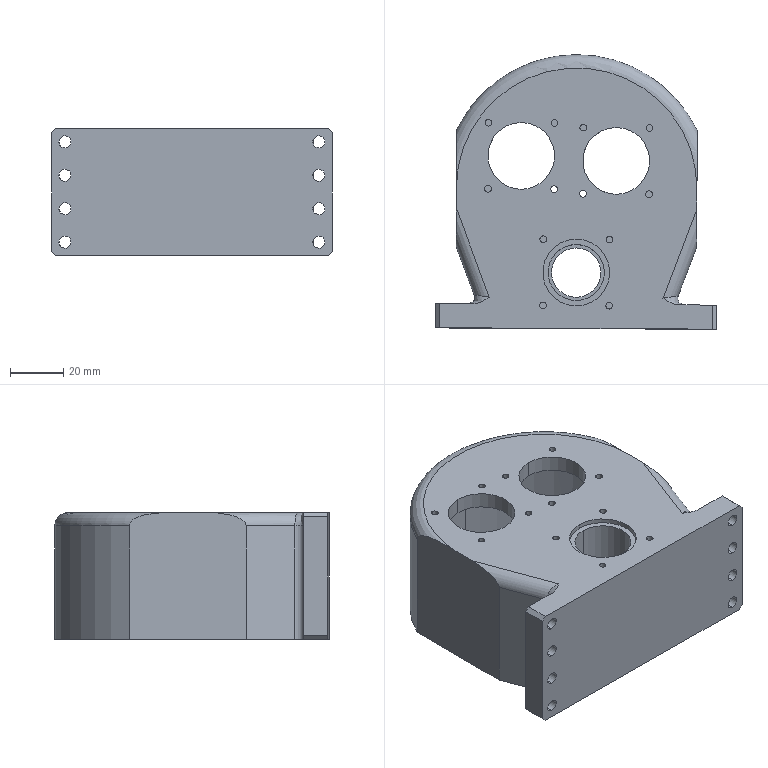Part | STEP file | 2026.6.15-Main Assembly图.sldasm-Part-129 | 1 solid | 141 faces | box 105.045 x 102.69 x 47.501 mm | volume 174792 mm3 | cylinder 87 | plane 45 | torus 7 | spline 2 | commonest cylinder face diameters 2.5 x24 3 x21 4.5 x16 25 x6 5 x5 20 x3